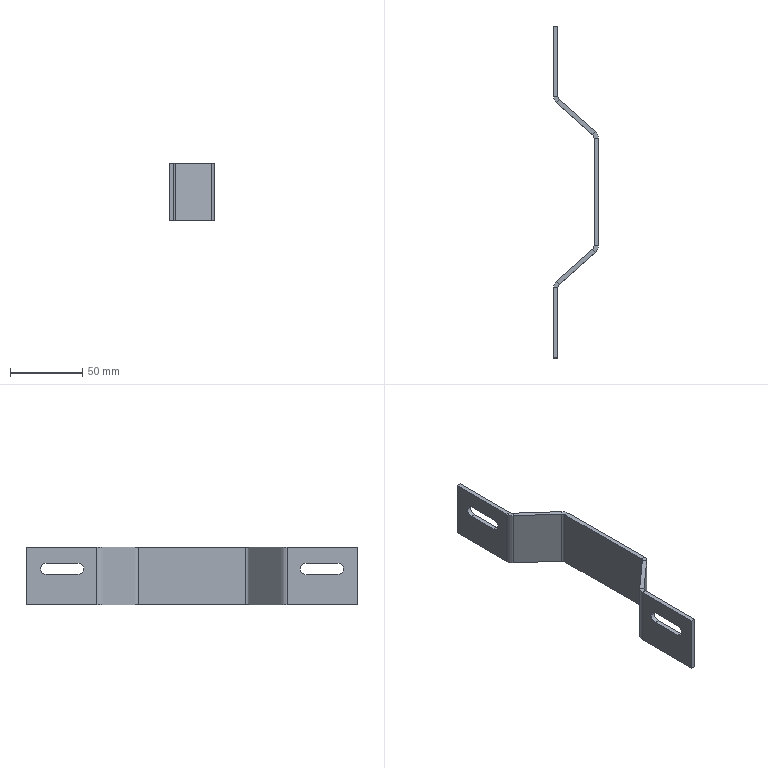Part | STEP file | 05-Switch striker | 1 solid | 48 faces | box 31 x 230 x 40 mm | volume 29136 mm3 | plane 34 | cylinder 14 | commonest cylinder face diameters 8 x6 6 x4 12 x4